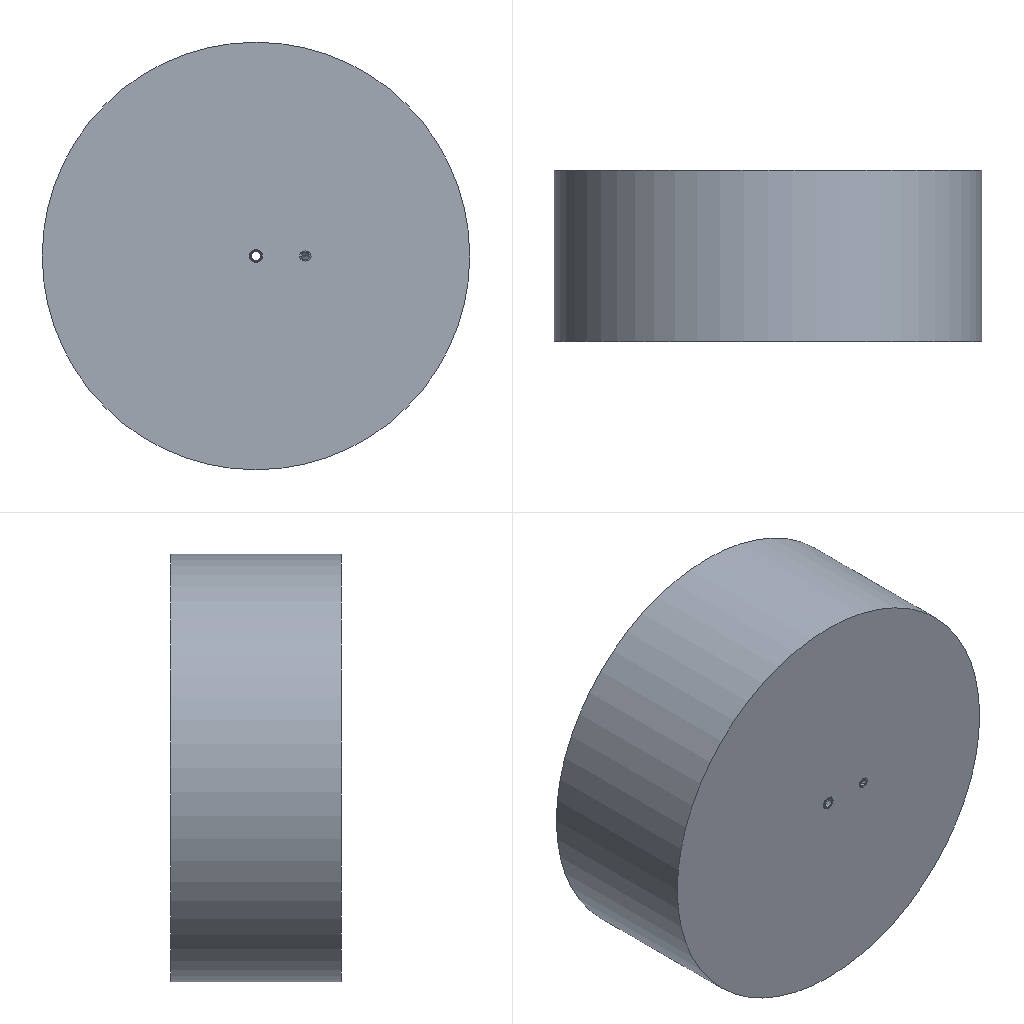Simulation study | abaqus
Set-up summary:
category,name,step,type,value,unit,region
solver,abaqus
solver,version,,,Abaqus/Standard 2020
units,not stated in the deck,,not stated
analysis,deck,,thermal,thermal
load_step,Step-1,Step-1,thermal
load_step,Step-2,Step-2,thermal
load_step,requested,,,2
mesh,nodes,,,40658
mesh,elements,,,93989
element_type,DC3D4,,solid,80589
element_type,DC3D8,,solid,13400
load,load commands in deck,,count,2
bc,support commands in deck,,count,1
material,CEMENT,,in results
material,COH,,in results
material,SOIL,,in results
material,TUBE,,in results
check,setup vs results,,match,"per instance, exact: element labels, types and connectivity; labels of the nodes the elements use; coordinates not compared"
Abaqus input file, long lists of numbers shortened:
*Heading
** Job name: TTT Model name: Model-1-Copy-Copy-TT
** Generated by: Abaqus/CAE 2020
*Preprint, echo=NO, model=NO, history=NO, contact=NO
**
** PARTS
**
*Part, name=P21
*Node
      1,   1050.777,           0.,           0.
      2,   1258.624,           0.,           0.
** (8455 more lines like these left out)
*Element, type=DC3D4
    1, 7574, 7583, 3286, 7573
    2, 7581, 3288, 3287, 3349
** (25295 more lines like these left out)
*Nset, nset=Set-1, generate
    1,  8457,     1
*Elset, elset=Set-1, generate
     1,  25297,      1
** Section: tube
*Solid Section, elset=Set-1, material=tube
,
*End Part
**
*Part, name=P22
*Node
      1,  -90.683,        4000.,   89.94
      2,           0.,        4000.,   155.24
** (1216 more lines like these left out)
*Element, type=DC3D4
   1, 1083,  994, 1100, 1016
   2, 1083, 1101,  994,  993
** (3592 more lines like these left out)
*Nset, nset=Set-1, generate
    1,  1218,     1
*Elset, elset=Set-1, generate
    1,  3594,     1
*Nset, nset=Set-2, generate
    1,  1218,     1
*Elset, elset=Set-2, generate
    1,  3594,     1
** Section: cement
*Solid Section, elset=Set-2, material=cement
,
*End Part
**
*Part, name=P23
*Node
      1,           0.,           0.,        5000.
      2,           0.,           0.,       -5000.
** (9675 more lines like these left out)
*Element, type=DC3D4
    1, 2201, 2202, 2203, 2204
    2, 2201, 2202, 2205, 2203
** (51696 more lines like these left out)
*Nset, nset=Set-1, generate
    1,  9677,     1
*Elset, elset=Set-1, generate
     1,  51698,      1
** Section: soil
*Solid Section, elset=Set-1, material=soil
,
*End Part
**
*Part, name=coh
*Node
      1,   112.261,  -48.373,           0.
      2,   121.754,   10.888,           0.
** (21304 more lines like these left out)
*Element, type=DC3D8
    1,   118,   131,   130,   176,    12,    25,    24,    70
    2,   149,   130,   131,   177,    43,    24,    25,    71
** (13398 more lines like these left out)
*Nset, nset=Set-2, generate
     1,  21306,      1
*Elset, elset=Set-2, generate
     1,  13400,      1
*Nset, nset=Set-7, generate
     1,  21306,      1
*Elset, elset=Set-7, generate
     1,  13400,      1
** Section: cement
*Solid Section, elset=Set-7, material=cement
,
*End Part
**
**
** ASSEMBLY
**
*Assembly, name=Assembly
**
*Instance, name=P21-1, part=P21
*End Instance
**
*Instance, name=P22-1, part=P22
*End Instance
**
*Instance, name=P23-1, part=P23
          0.,        4000.,           0.
          0.,        4000.,           0.,           1.,        4000., 6.12323426292584e-17,         180.
*End Instance
**
*Instance, name=coh-1, part=coh
          0.,           0.,           0.
          0.,           0.,           0., -1.,           0.,           0., 90.
*End Instance
**
*Nset, nset=Set-1, instance=P21-1
   1,   2,   3,   4,   9,  10,  11,  12,  17,  18,  19,  20,  21,  22,  23,  24
  25,  26,  27,  28,  29,  30,  31,  32,  33,  34,  35,  36,  37,  38,  39,  40
** (4 more lines like these left out)
*Nset, nset=Set-1, instance=P22-1
  10,  11,  12,  13, 135, 136, 137, 138, 139, 140, 163, 164, 165, 166, 167, 168
*Nset, nset=Set-1, instance=P23-1
    5,    6,    9,   10,   11,   12,   88,   89,   90,   91,   92,   93,  112,  113,  114,  115
  116,  117,  124,  125,  126,  127,  128,  129,  130,  131,  132,  133,  134,  135,  136,  137
** (53 more lines like these left out)
*Elset, elset=Set-1, instance=P21-1
   838,   844,   850,   902,   938,  1491,  6031, 10297, 10301, 10312, 10314, 10326, 10328, 10341, 10342, 10361
 10389, 10392, 10394, 10405, 10420, 10436, 10440, 10451, 10465, 10466, 10468, 10473, 10474, 10481, 10482, 10487
** (4 more lines like these left out)
*Elset, elset=Set-1, instance=P22-1
  137,  140,  149,  150,  172,  563,  564,  723,  740,  744,  752,  777,  789,  797,  836, 1811
*Elset, elset=Set-1, instance=P23-1
    15,   152,   213,   350,   508,   532,   550,   619,   665,   831,  1279,  1311,  1422,  1458,  1522,  1597
  1651,  1745,  1796,  1807,  1938,  2013,  2113,  2181,  2314,  2352,  2353,  2435,  2530,  2604,  2626,  2627
** (103 more lines like these left out)
*Nset, nset=Set-2, instance=P21-1, generate
    1,  8457,     1
*Nset, nset=Set-2, instance=P22-1, generate
    1,  1218,     1
*Nset, nset=Set-2, instance=P23-1, generate
    1,  9677,     1
*Elset, elset=Set-2, instance=P21-1, generate
     1,  25297,      1
*Elset, elset=Set-2, instance=P22-1, generate
    1,  3594,     1
*Elset, elset=Set-2, instance=P23-1, generate
     1,  51698,      1
*Nset, nset=Set-3, instance=P21-1, generate
    1,  8457,     1
*Nset, nset=Set-3, instance=P22-1, generate
    1,  1218,     1
*Nset, nset=Set-3, instance=P23-1, generate
    1,  9677,     1
*Elset, elset=Set-3, instance=P21-1, generate
     1,  25297,      1
*Elset, elset=Set-3, instance=P22-1, generate
    1,  3594,     1
*Elset, elset=Set-3, instance=P23-1, generate
     1,  51698,      1
*Nset, nset=Set-4, instance=P21-1, generate
    1,  8457,     1
*Nset, nset=Set-4, instance=P22-1, generate
    1,  1218,     1
*Nset, nset=Set-4, instance=P23-1, generate
    1,  9677,     1
*Elset, elset=Set-4, instance=P21-1, generate
     1,  25297,      1
*Elset, elset=Set-4, instance=P22-1, generate
    1,  3594,     1
*Elset, elset=Set-4, instance=P23-1, generate
     1,  51698,      1
*Nset, nset=Set-5, instance=P21-1, generate
    1,  8457,     1
*Nset, nset=Set-5, instance=P22-1, generate
    1,  1218,     1
*Nset, nset=Set-5, instance=P23-1, generate
    1,  9677,     1
*Nset, nset=Set-5, instance=coh-1, generate
     1,  21306,      1
*Elset, elset=Set-5, instance=P21-1, generate
     1,  25297,      1
*Elset, elset=Set-5, instance=P22-1, generate
    1,  3594,     1
*Elset, elset=Set-5, instance=P23-1, generate
     1,  51698,      1
*Elset, elset=Set-5, instance=coh-1, generate
     1,  13400,      1
*Elset, elset=_Surf-1_S3, internal, instance=P21-1
     2,     3,     8,    15,    31,    34,    47,    52,    72,    76,    84,    95,    96,   102,   110,   123
   124,   147,   149,   153,   177,   183,   185,   186,   189,   202,   206,   207,   217,   228,   235,   245
** (439 more lines like these left out)
*Elset, elset=_Surf-1_S4, internal, instance=P21-1
    29,    37,   119,   143,   154,   167,   325,   397,   465,   499,   565,   610,   652,   667,   673,   718
   773,   838,   844,   864,   913,   920,   938,   945,   955,   966,   992,  1009,  1011,  1015,  1066,  1087
** (22 more lines like these left out)
*Elset, elset=_Surf-1_S1, internal, instance=P21-1
   223,   420,   443,   459,   693,   785,   830,   866,  1608,  1623,  2301,  2526,  3215,  3218,  3593,  3598
  3692,  4192,  4402,  4443,  4547,  4582,  4586,  4798,  5314,  5372,  5657,  5929,  6073,  6639,  6643,  7053
** (13 more lines like these left out)
*Elset, elset=_Surf-1_S2, internal, instance=P21-1
    21,    54,   273,   331,   336,   367,   449,   491,   522,   543,   612,   653,   655,   658,  1065,  1111
  1139,  1180,  1261,  1290,  1705,  2255,  2774,  2778,  2863,  3034,  3327,  3662,  4244,  4304,  4344,  4485
** (16 more lines like these left out)
*Surface, type=ELEMENT, name=Surf-1
_Surf-1_S3, S3
_Surf-1_S4, S4
_Surf-1_S2, S2
_Surf-1_S1, S1
*Elset, elset=_Surf-2_S4, internal, instance=P21-1
    11,    13,    26,    29,    37,    38,    58,    59,    78,    88,    93,   112,   119,   122,   127,   143
   145,   154,   159,   167,   171,   174,   187,   190,   196,   199,   212,   243,   262,   285,   297,   300
** (158 more lines like these left out)
*Elset, elset=_Surf-2_S4, internal, instance=P22-1
   10,   13,   15,   19,   21,   29,   64,   82,   86,   93,   99,  103,  106,  110,  121,  128
  143,  156,  160,  165,  170,  174,  200,  231,  238,  243,  245,  254,  262,  263,  269,  272
** (16 more lines like these left out)
*Elset, elset=_Surf-2_S4, internal, instance=P23-1
   293,  1215,  1422,  1704,  2620,  2635,  2721,  2737,  2758,  2882,  2966,  3146,  3160,  3288,  3450,  3914
  4023,  4055,  4489,  4644,  4717,  4811,  4903,  5114,  5203,  5349,  5376,  5379,  5392,  5576,  5614,  5738
** (8 more lines like these left out)
*Elset, elset=_Surf-2_S2, internal, instance=P21-1
     1,     7,    12,    21,    23,    27,    35,    54,    56,    66,    67,    74,    77,    90,    94,    99
   105,   116,   125,   131,   134,   135,   140,   144,   156,   160,   161,   168,   178,   181,   184,   191
** (204 more lines like these left out)
*Elset, elset=_Surf-2_S2, internal, instance=P22-1
    3,   14,   26,   39,   44,   51,   53,   60,   66,   68,   72,   85,   92,  102,  104,  109
  122,  127,  129,  134,  137,  140,  144,  149,  155,  158,  172,  176,  177,  179,  189,  204
** (25 more lines like these left out)
*Elset, elset=_Surf-2_S2, internal, instance=P23-1
    15,   213,  1425,  2671,  2680,  2681,  2697,  2946,  3058,  3136,  3248,  3276,  3288,  3625,  3774,  3778
  3922,  4321,  4378,  4380,  4426,  4580,  4736,  4740,  4848,  4913,  5018,  5098,  5140,  5172,  5368,  5369
** (10 more lines like these left out)
*Elset, elset=_Surf-2_S1, internal, instance=P21-1
    17,    18,    19,    28,    42,    45,    46,    48,    57,    63,    71,    73,    79,    80,    82,    89
   100,   104,   111,   113,   117,   120,   136,   137,   150,   169,   173,   188,   193,   194,   197,   201
** (219 more lines like these left out)
*Elset, elset=_Surf-2_S1, internal, instance=P22-1
    4,    7,   20,   27,   30,   32,   33,   69,   75,   76,   77,   81,  101,  113,  116,  123
  131,  135,  137,  149,  150,  159,  163,  168,  178,  181,  182,  184,  186,  192,  201,  209
** (24 more lines like these left out)
*Elset, elset=_Surf-2_S1, internal, instance=P23-1
  2647,  2650,  2681,  2737,  4903,  5051,  5114,  5379,  5562,  5942,  5948,  5991,  6048,  6147,  6285,  6327
  6728,  6913,  7548,  7761,  7950,  7962,  8070,  8084,  8120,  8147,  8159,  8448,  8627,  8801,  8819,  8866
** (6 more lines like these left out)
*Elset, elset=_Surf-2_S3, internal, instance=P21-1
     2,     3,     8,    15,    31,    34,    47,    52,    72,    76,    84,    85,    95,    96,   102,   106
   108,   110,   123,   124,   141,   147,   149,   153,   175,   177,   183,   185,   186,   189,   202,   206
** (467 more lines like these left out)
*Elset, elset=_Surf-2_S3, internal, instance=P22-1
   24,   43,   73,  118,  164,  196,  240,  310,  343,  368,  376,  385,  406,  423,  430,  499
  564,  581,  727,  735,  752,  797,  849,  881,  956, 1048, 1196, 1213, 1256, 1265, 1315, 1330
** (3 more lines like these left out)
*Elset, elset=_Surf-2_S3, internal, instance=P23-1
    27,    30,    53,    61,    90,   113,   114,   152,   174,   210,   218,   350,   398,   498,   502,   503
   508,   532,   550,   619,   665,   741,   831,   847,   928,  1058,  1143,  1209,  1243,  1279,  1311,  1319
** (245 more lines like these left out)
*Surface, type=ELEMENT, name=Surf-2
_Surf-2_S4, S4
_Surf-2_S2, S2
_Surf-2_S1, S1
_Surf-2_S3, S3
*Elset, elset=_Surf-3_S4, internal, instance=P21-1
    11,    13,    26,    29,    37,    38,    58,    59,    78,    88,    93,   112,   119,   122,   127,   143
   145,   154,   159,   167,   171,   174,   187,   190,   196,   199,   212,   243,   262,   285,   297,   300
** (158 more lines like these left out)
*Elset, elset=_Surf-3_S4, internal, instance=P22-1
   10,   13,   15,   19,   21,   29,   64,   82,   86,   93,   99,  103,  106,  110,  121,  128
  143,  156,  160,  165,  170,  174,  200,  231,  238,  243,  245,  254,  262,  263,  269,  272
** (16 more lines like these left out)
*Elset, elset=_Surf-3_S4, internal, instance=P23-1
   293,  1215,  1422,  1704,  2620,  2635,  2721,  2737,  2758,  2882,  2966,  3146,  3160,  3288,  3450,  3914
  4023,  4055,  4489,  4644,  4717,  4811,  4903,  5114,  5203,  5349,  5376,  5379,  5392,  5576,  5614,  5738
** (8 more lines like these left out)
*Elset, elset=_Surf-3_S2, internal, instance=P21-1
     1,     7,    12,    21,    23,    27,    35,    54,    56,    66,    67,    74,    77,    90,    94,    99
   105,   116,   125,   131,   134,   135,   140,   144,   156,   160,   161,   168,   178,   181,   184,   191
** (204 more lines like these left out)
*Elset, elset=_Surf-3_S2, internal, instance=P22-1
    3,   14,   26,   39,   44,   51,   53,   60,   66,   68,   72,   85,   92,  102,  104,  109
  122,  127,  129,  134,  137,  140,  144,  149,  155,  158,  172,  176,  177,  179,  189,  204
** (25 more lines like these left out)
*Elset, elset=_Surf-3_S2, internal, instance=P23-1
    15,   213,  1425,  2671,  2680,  2681,  2697,  2946,  3058,  3136,  3248,  3276,  3288,  3625,  3774,  3778
  3922,  4321,  4378,  4380,  4426,  4580,  4736,  4740,  4848,  4913,  5018,  5098,  5140,  5172,  5368,  5369
** (10 more lines like these left out)
*Elset, elset=_Surf-3_S1, internal, instance=P21-1
    17,    18,    19,    28,    42,    45,    46,    48,    57,    63,    71,    73,    79,    80,    82,    89
   100,   104,   111,   113,   117,   120,   136,   137,   150,   169,   173,   188,   193,   194,   197,   201
** (219 more lines like these left out)
*Elset, elset=_Surf-3_S1, internal, instance=P22-1
    4,    7,   20,   27,   30,   32,   33,   69,   75,   76,   77,   81,  101,  113,  116,  123
  131,  135,  137,  149,  150,  159,  163,  168,  178,  181,  182,  184,  186,  192,  201,  209
** (24 more lines like these left out)
*Elset, elset=_Surf-3_S1, internal, instance=P23-1
  2647,  2650,  2681,  2737,  4903,  5051,  5114,  5379,  5562,  5942,  5948,  5991,  6048,  6147,  6285,  6327
  6728,  6913,  7548,  7761,  7950,  7962,  8070,  8084,  8120,  8147,  8159,  8448,  8627,  8801,  8819,  8866
** (6 more lines like these left out)
*Elset, elset=_Surf-3_S3, internal, instance=P21-1
     2,     3,     8,    15,    31,    34,    47,    52,    72,    76,    84,    85,    95,    96,   102,   106
   108,   110,   123,   124,   141,   147,   149,   153,   175,   177,   183,   185,   186,   189,   202,   206
** (467 more lines like these left out)
*Elset, elset=_Surf-3_S3, internal, instance=P22-1
   24,   43,   73,  118,  164,  196,  240,  310,  343,  368,  376,  385,  406,  423,  430,  499
  564,  581,  727,  735,  752,  797,  849,  881,  956, 1048, 1196, 1213, 1256, 1265, 1315, 1330
** (3 more lines like these left out)
*Elset, elset=_Surf-3_S3, internal, instance=P23-1
    27,    30,    53,    61,    90,   113,   114,   152,   174,   210,   218,   350,   398,   498,   502,   503
   508,   532,   550,   619,   665,   741,   831,   847,   928,  1058,  1143,  1209,  1243,  1279,  1311,  1319
** (245 more lines like these left out)
*Surface, type=ELEMENT, name=Surf-3
_Surf-3_S4, S4
_Surf-3_S2, S2
_Surf-3_S1, S1
_Surf-3_S3, S3
*Elset, elset=_Surf-14_S4, internal, instance=P21-1
    11,    13,    26,    29,    37,    38,    58,    59,    78,    88,    93,   112,   119,   122,   127,   143
   145,   154,   159,   167,   171,   174,   187,   190,   196,   199,   212,   243,   262,   285,   297,   300
** (158 more lines like these left out)
*Elset, elset=_Surf-14_S4, internal, instance=P22-1
   10,   13,   15,   19,   21,   29,   38,   47,   64,   71,   82,   86,   93,   99,  103,  106
  110,  121,  128,  143,  156,  160,  165,  166,  167,  169,  170,  174,  175,  190,  200,  207
** (25 more lines like these left out)
*Elset, elset=_Surf-14_S4, internal, instance=P23-1
   293,  1215,  1422,  1704,  2620,  2635,  2721,  2737,  2758,  2882,  2966,  3146,  3160,  3288,  3450,  3914
  4023,  4055,  4489,  4644,  4717,  4811,  4903,  5114,  5203,  5349,  5376,  5379,  5392,  5576,  5614,  5738
** (8 more lines like these left out)
*Elset, elset=_Surf-14_S4, internal, instance=coh-1
     4,     9,    10,    14,    15,    18,    19,    20,    25,    26,    30,    31,    32,    33,    39,    52
    59,    63,    64,    71,    76,    77,    81,    82,    85,    86,    87,    92,    93,    97,    98,    99
** (236 more lines like these left out)
*Elset, elset=_Surf-14_S2, internal, instance=P21-1
     1,     7,    12,    21,    23,    27,    35,    54,    56,    66,    67,    74,    77,    90,    94,    99
   105,   116,   125,   131,   134,   135,   140,   144,   156,   160,   161,   168,   178,   181,   184,   191
** (204 more lines like these left out)
*Elset, elset=_Surf-14_S2, internal, instance=P22-1
    3,   14,   18,   26,   39,   44,   51,   53,   60,   66,   68,   72,   80,   85,   92,  102
  104,  109,  122,  127,  129,  134,  137,  140,  144,  149,  155,  158,  172,  176,  177,  179
** (31 more lines like these left out)
*Elset, elset=_Surf-14_S2, internal, instance=P23-1
    15,   213,  1425,  2671,  2680,  2681,  2697,  2946,  3058,  3136,  3248,  3276,  3288,  3625,  3774,  3778
  3922,  4321,  4378,  4380,  4426,  4580,  4736,  4740,  4848,  4913,  5018,  5098,  5140,  5172,  5368,  5369
** (10 more lines like these left out)
*Elset, elset=_Surf-14_S2, internal, instance=coh-1, generate
  1,  67,   1
*Elset, elset=_Surf-14_S1, internal, instance=P21-1
    17,    18,    19,    28,    42,    45,    46,    48,    57,    63,    71,    73,    79,    80,    82,    89
   100,   104,   111,   113,   117,   120,   136,   137,   150,   169,   173,   188,   193,   194,   197,   201
** (219 more lines like these left out)
*Elset, elset=_Surf-14_S1, internal, instance=P22-1
    4,    7,   20,   27,   30,   32,   33,   63,   69,   75,   76,   77,   81,  101,  113,  116
  123,  131,  135,  137,  149,  150,  159,  163,  168,  178,  181,  182,  184,  185,  186,  192
** (29 more lines like these left out)
*Elset, elset=_Surf-14_S1, internal, instance=P23-1
  2647,  2650,  2681,  2737,  4903,  5051,  5114,  5379,  5562,  5942,  5948,  5991,  6048,  6147,  6285,  6327
  6728,  6913,  7548,  7761,  7950,  7962,  8070,  8084,  8120,  8147,  8159,  8448,  8627,  8801,  8819,  8866
** (6 more lines like these left out)
*Elset, elset=_Surf-14_S1, internal, instance=coh-1, generate
 13334,  13400,      1
*Elset, elset=_Surf-14_S3, internal, instance=P21-1
     2,     3,     8,    15,    31,    34,    47,    52,    72,    76,    84,    85,    95,    96,   102,   106
   108,   110,   123,   124,   141,   147,   149,   153,   175,   177,   183,   185,   186,   189,   202,   206
** (467 more lines like these left out)
*Elset, elset=_Surf-14_S3, internal, instance=P22-1
   24,   34,   41,   43,   52,   56,   57,   58,   65,   67,   73,   94,   95,   98,  105,  112
  118,  120,  138,  161,  164,  180,  194,  195,  196,  219,  233,  236,  240,  244,  249,  250
** (62 more lines like these left out)
*Elset, elset=_Surf-14_S3, internal, instance=P23-1
    27,    30,    53,    61,    90,   113,   114,   152,   174,   210,   218,   350,   398,   498,   502,   503
   508,   532,   550,   619,   665,   741,   831,   847,   928,  1058,  1143,  1209,  1243,  1279,  1311,  1319
** (245 more lines like these left out)
*Elset, elset=_Surf-14_S3, internal, instance=coh-1
     1,     2,     6,    11,    12,    13,    22,    34,    38,    40,    41,    42,    43,    47,    48,    53
    54,    56,    57,    68,    69,    73,    78,    79,    80,    89,   101,   105,   107,   108,   109,   110
** (236 more lines like these left out)
*Elset, elset=_Surf-14_S5, internal, instance=coh-1
     1,     2,     5,     8,    11,    12,    13,    16,    17,    27,    28,    34,    35,    36,    44,    45
    47,    48,    49,    67,    68,    69,    72,    75,    78,    79,    80,    83,    84,    94,    95,   101
** (248 more lines like these left out)
*Elset, elset=_Surf-14_S6, internal, instance=coh-1
     7,     9,    10,    14,    15,    21,    23,    24,    29,    31,    32,    33,    37,    46,    50,    51
    55,    61,    65,    66,    74,    76,    77,    81,    82,    88,    90,    91,    96,    98,    99,   100
** (248 more lines like these left out)
*Surface, type=ELEMENT, name=Surf-14
_Surf-14_S4, S4
_Surf-14_S2, S2
_Surf-14_S6, S6
_Surf-14_S1, S1
_Surf-14_S3, S3
_Surf-14_S5, S5
*Elset, elset=_Surf-15_S4, internal, instance=P21-1
    11,    13,    26,    29,    37,    38,    58,    59,    78,    88,    93,   112,   119,   122,   127,   143
   145,   154,   159,   167,   171,   174,   187,   190,   196,   199,   212,   243,   262,   285,   297,   300
** (158 more lines like these left out)
*Elset, elset=_Surf-15_S4, internal, instance=P22-1
   10,   13,   15,   19,   21,   29,   38,   47,   64,   71,   82,   86,   93,   99,  103,  106
  110,  121,  128,  143,  156,  160,  165,  166,  167,  169,  170,  174,  175,  190,  200,  207
** (25 more lines like these left out)
*Elset, elset=_Surf-15_S4, internal, instance=P23-1
   293,  1215,  1422,  1704,  2620,  2635,  2721,  2737,  2758,  2882,  2966,  3146,  3160,  3288,  3450,  3914
  4023,  4055,  4489,  4644,  4717,  4811,  4903,  5114,  5203,  5349,  5376,  5379,  5392,  5576,  5614,  5738
** (8 more lines like these left out)
*Elset, elset=_Surf-15_S4, internal, instance=coh-1
     4,     9,    10,    14,    15,    18,    19,    20,    25,    26,    30,    31,    32,    33,    39,    52
    59,    63,    64,    71,    76,    77,    81,    82,    85,    86,    87,    92,    93,    97,    98,    99
** (236 more lines like these left out)
*Elset, elset=_Surf-15_S2, internal, instance=P21-1
     1,     7,    12,    21,    23,    27,    35,    54,    56,    66,    67,    74,    77,    90,    94,    99
   105,   116,   125,   131,   134,   135,   140,   144,   156,   160,   161,   168,   178,   181,   184,   191
** (204 more lines like these left out)
*Elset, elset=_Surf-15_S2, internal, instance=P22-1
    3,   14,   18,   26,   39,   44,   51,   53,   60,   66,   68,   72,   80,   85,   92,  102
  104,  109,  122,  127,  129,  134,  137,  140,  144,  149,  155,  158,  172,  176,  177,  179
** (31 more lines like these left out)
*Elset, elset=_Surf-15_S2, internal, instance=P23-1
    15,   213,  1425,  2671,  2680,  2681,  2697,  2946,  3058,  3136,  3248,  3276,  3288,  3625,  3774,  3778
  3922,  4321,  4378,  4380,  4426,  4580,  4736,  4740,  4848,  4913,  5018,  5098,  5140,  5172,  5368,  5369
** (10 more lines like these left out)
*Elset, elset=_Surf-15_S2, internal, instance=coh-1, generate
  1,  67,   1
*Elset, elset=_Surf-15_S1, internal, instance=P21-1
    17,    18,    19,    28,    42,    45,    46,    48,    57,    63,    71,    73,    79,    80,    82,    89
   100,   104,   111,   113,   117,   120,   136,   137,   150,   169,   173,   188,   193,   194,   197,   201
** (219 more lines like these left out)
*Elset, elset=_Surf-15_S1, internal, instance=P22-1
    4,    7,   20,   27,   30,   32,   33,   63,   69,   75,   76,   77,   81,  101,  113,  116
  123,  131,  135,  137,  149,  150,  159,  163,  168,  178,  181,  182,  184,  185,  186,  192
** (29 more lines like these left out)
*Elset, elset=_Surf-15_S1, internal, instance=P23-1
  2647,  2650,  2681,  2737,  4903,  5051,  5114,  5379,  5562,  5942,  5948,  5991,  6048,  6147,  6285,  6327
  6728,  6913,  7548,  7761,  7950,  7962,  8070,  8084,  8120,  8147,  8159,  8448,  8627,  8801,  8819,  8866
** (6 more lines like these left out)
*Elset, elset=_Surf-15_S1, internal, instance=coh-1, generate
 13334,  13400,      1
*Elset, elset=_Surf-15_S3, internal, instance=P21-1
     2,     3,     8,    15,    31,    34,    47,    52,    72,    76,    84,    85,    95,    96,   102,   106
   108,   110,   123,   124,   141,   147,   149,   153,   175,   177,   183,   185,   186,   189,   202,   206
** (467 more lines like these left out)
*Elset, elset=_Surf-15_S3, internal, instance=P22-1
   24,   34,   41,   43,   52,   56,   57,   58,   65,   67,   73,   94,   95,   98,  105,  112
  118,  120,  138,  161,  164,  180,  194,  195,  196,  219,  233,  236,  240,  244,  249,  250
** (62 more lines like these left out)
*Elset, elset=_Surf-15_S3, internal, instance=P23-1
    27,    30,    53,    61,    90,   113,   114,   152,   174,   210,   218,   350,   398,   498,   502,   503
   508,   532,   550,   619,   665,   741,   831,   847,   928,  1058,  1143,  1209,  1243,  1279,  1311,  1319
** (245 more lines like these left out)
*Elset, elset=_Surf-15_S3, internal, instance=coh-1
     1,     2,     6,    11,    12,    13,    22,    34,    38,    40,    41,    42,    43,    47,    48,    53
    54,    56,    57,    68,    69,    73,    78,    79,    80,    89,   101,   105,   107,   108,   109,   110
** (236 more lines like these left out)
*Elset, elset=_Surf-15_S5, internal, instance=coh-1
     1,     2,     5,     8,    11,    12,    13,    16,    17,    27,    28,    34,    35,    36,    44,    45
    47,    48,    49,    67,    68,    69,    72,    75,    78,    79,    80,    83,    84,    94,    95,   101
** (248 more lines like these left out)
*Elset, elset=_Surf-15_S6, internal, instance=coh-1
     7,     9,    10,    14,    15,    21,    23,    24,    29,    31,    32,    33,    37,    46,    50,    51
    55,    61,    65,    66,    74,    76,    77,    81,    82,    88,    90,    91,    96,    98,    99,   100
** (248 more lines like these left out)
*Surface, type=ELEMENT, name=Surf-15
_Surf-15_S4, S4
_Surf-15_S2, S2
_Surf-15_S6, S6
_Surf-15_S1, S1
_Surf-15_S3, S3
_Surf-15_S5, S5
*Elset, elset=_m_Surf-4_S2, internal, instance=P21-1
     1,     7,    12,    23,    27,    35,    56,    66,    67,    74,    77,    90,    94,    99,   105,   116
   125,   131,   134,   135,   140,   144,   156,   160,   161,   168,   178,   181,   184,   191,   215,   216
** (137 more lines like these left out)
*Elset, elset=_m_Surf-4_S4, internal, instance=P21-1
    11,    13,    26,    38,    58,    78,    88,    93,   112,   122,   127,   145,   159,   171,   174,   187
   190,   196,   199,   212,   243,   262,   285,   297,   300,   316,   337,   344,   352,   378,   390,   404
** (90 more lines like these left out)
*Elset, elset=_m_Surf-4_S1, internal, instance=P21-1
    17,    18,    19,    28,    42,    45,    46,    48,    57,    63,    71,    73,    79,    80,    82,    89
   100,   104,   111,   113,   117,   120,   136,   137,   150,   169,   173,   188,   193,   194,   197,   201
** (148 more lines like these left out)
*Elset, elset=_m_Surf-4_S3, internal, instance=P21-1
    85,   106,   108,   141,   175,   211,   272,   345,   348,   368,   376,   417,   462,   471,   492,   498
   550,   551,   554,   564,   615,   640,   661,   682,   687,   735,   765,   803,   811,   889,   901,   915
** (17 more lines like these left out)
*Surface, type=ELEMENT, name=m_Surf-4
_m_Surf-4_S2, S2
_m_Surf-4_S4, S4
_m_Surf-4_S1, S1
_m_Surf-4_S3, S3
*Elset, elset=_m_Surf-6_S4, internal, instance=P22-1
   64,  480,  490,  496,  497,  672,  832, 1112, 1114, 1197, 1198, 1222, 1229, 1233, 1235, 1237
 1248, 1305, 1312, 1316, 1332, 1344, 1401, 1406, 1435, 1446, 1448, 1450, 1480, 1501, 1570, 1578
** (10 more lines like these left out)
*Elset, elset=_m_Surf-6_S2, internal, instance=P22-1
  102,  446,  771,  792,  923,  983, 1188, 1193, 1195, 1200, 1204, 1206, 1212, 1216, 1236, 1249
 1250, 1258, 1268, 1269, 1274, 1282, 1283, 1284, 1294, 1295, 1300, 1314, 1318, 1325, 1339, 1340
** (16 more lines like these left out)
*Elset, elset=_m_Surf-6_S3, internal, instance=P22-1
  423,  727,  849, 1196, 1256, 1265, 1315, 1330, 1343, 1752, 1758, 1792, 1884, 1888, 1892, 1895
 1936, 1947, 2008, 2011, 2226, 2297, 2342, 2357, 2565, 2574, 2575, 2586, 2587, 2610, 2632, 2688
** (1 more lines like these left out)
*Elset, elset=_m_Surf-6_S1, internal, instance=P22-1
  489,  844, 1202, 1211, 1220, 1221, 1227, 1231, 1241, 1245, 1255, 1261, 1264, 1270, 1273, 1285
 1287, 1288, 1290, 1297, 1298, 1306, 1317, 1320, 1326, 1331, 1334, 1335, 1348, 1349, 1361, 1364
** (16 more lines like these left out)
*Surface, type=ELEMENT, name=m_Surf-6
_m_Surf-6_S4, S4
_m_Surf-6_S2, S2
_m_Surf-6_S3, S3
_m_Surf-6_S1, S1
*Elset, elset=_m_Surf-8_S2, internal, instance=P21-1
     1,     7,    12,    23,    27,    35,    56,    66,    67,    74,    77,    90,    94,    99,   105,   116
   125,   131,   134,   135,   140,   144,   156,   160,   161,   168,   178,   181,   184,   191,   215,   216
** (137 more lines like these left out)
*Elset, elset=_m_Surf-8_S4, internal, instance=P21-1
    11,    13,    26,    38,    58,    78,    88,    93,   112,   122,   127,   145,   159,   171,   174,   187
   190,   196,   199,   212,   243,   262,   285,   297,   300,   316,   337,   344,   352,   378,   390,   404
** (90 more lines like these left out)
*Elset, elset=_m_Surf-8_S1, internal, instance=P21-1
    17,    18,    19,    28,    42,    45,    46,    48,    57,    63,    71,    73,    79,    80,    82,    89
   100,   104,   111,   113,   117,   120,   136,   137,   150,   169,   173,   188,   193,   194,   197,   201
** (148 more lines like these left out)
*Elset, elset=_m_Surf-8_S3, internal, instance=P21-1
    85,   106,   108,   141,   175,   211,   272,   345,   348,   368,   376,   417,   462,   471,   492,   498
   550,   551,   554,   564,   615,   640,   661,   682,   687,   735,   765,   803,   811,   889,   901,   915
** (17 more lines like these left out)
*Surface, type=ELEMENT, name=m_Surf-8
_m_Surf-8_S2, S2
_m_Surf-8_S4, S4
_m_Surf-8_S1, S1
_m_Surf-8_S3, S3
*Elset, elset=_m_Surf-10_S5, internal, instance=coh-1
     1,     5,     8,    11,    12,    13,    17,    27,    34,    49,    67,    68,    72,    75,    78,    79
    80,    84,    94,   101,   116,   134,   135,   139,   142,   145,   146,   147,   151,   161,   168,   183
** (136 more lines like these left out)
*Elset, elset=_m_Surf-10_S3, internal, instance=coh-1
     2,     6,    38,    47,    48,    56,    57,    69,    73,   105,   114,   115,   123,   124,   136,   140
   172,   181,   182,   190,   191,   203,   207,   239,   248,   249,   257,   258,   270,   274,   306,   315
** (86 more lines like these left out)
*Elset, elset=_m_Surf-10_S6, internal, instance=coh-1
     7,    10,    15,    23,    29,    31,    32,    37,    46,    51,    61,    74,    77,    82,    90,    96
    98,    99,   104,   113,   118,   128,   141,   144,   149,   157,   163,   165,   166,   171,   180,   185
** (136 more lines like these left out)
*Elset, elset=_m_Surf-10_S4, internal, instance=coh-1
     9,    14,    18,    19,    20,    26,    30,    33,    39,    52,    59,    76,    81,    85,    86,    87
    93,    97,   100,   106,   119,   126,   143,   148,   152,   153,   154,   160,   164,   167,   173,   186
** (136 more lines like these left out)
*Surface, type=ELEMENT, name=m_Surf-10
_m_Surf-10_S5, S5
_m_Surf-10_S3, S3
_m_Surf-10_S6, S6
_m_Surf-10_S4, S4
*Elset, elset=_m_Surf-12_S2, internal, instance=P21-1
     1,     7,    12,    23,    27,    35,    56,    66,    67,    74,    77,    90,    94,    99,   105,   116
   125,   131,   134,   135,   140,   144,   156,   160,   161,   168,   178,   181,   184,   191,   215,   216
** (137 more lines like these left out)
*Elset, elset=_m_Surf-12_S4, internal, instance=P21-1
    11,    13,    26,    38,    58,    78,    88,    93,   112,   122,   127,   145,   159,   171,   174,   187
   190,   196,   199,   212,   243,   262,   285,   297,   300,   316,   337,   344,   352,   378,   390,   404
** (90 more lines like these left out)
*Elset, elset=_m_Surf-12_S1, internal, instance=P21-1
    17,    18,    19,    28,    42,    45,    46,    48,    57,    63,    71,    73,    79,    80,    82,    89
   100,   104,   111,   113,   117,   120,   136,   137,   150,   169,   173,   188,   193,   194,   197,   201
** (148 more lines like these left out)
*Elset, elset=_m_Surf-12_S3, internal, instance=P21-1
    85,   106,   108,   141,   175,   211,   272,   345,   348,   368,   376,   417,   462,   471,   492,   498
   550,   551,   554,   564,   615,   640,   661,   682,   687,   735,   765,   803,   811,   889,   901,   915
** (17 more lines like these left out)
*Surface, type=ELEMENT, name=m_Surf-12
_m_Surf-12_S2, S2
_m_Surf-12_S4, S4
_m_Surf-12_S1, S1
_m_Surf-12_S3, S3
*Elset, elset=_s_Surf-6_S3, internal, instance=P23-1
   113,  2445,  2454,  2467,  2494,  2580,  2618,  2650,  2656,  2661,  2675,  2682,  2686,  2687,  2711,  2727
  2747,  2753,  2754,  2855,  2863,  2924,  2936,  3141,  3147,  3270,  3293,  3338,  3399,  3442,  3477,  3544
** (29 more lines like these left out)
*Elset, elset=_s_Surf-6_S2, internal, instance=P23-1
  2680,  3058,  3136,  3276,  6688,  6694,  7196,  7224,  7651,  7764,  7931,  7936,  7968,  8152,  8158,  8593
  9731, 11220, 11245, 11502, 16204, 17280
*Elset, elset=_s_Surf-6_S4, internal, instance=P23-1
  3160,  3288,  3450,  4055,  6539,  7704,  7827,  7836,  7940,  7977,  8310,  8312, 11229, 11293, 12046, 12974
 19345, 22350, 22855, 24051, 25027, 35622, 36049
*Elset, elset=_s_Surf-6_S1, internal, instance=P23-1
  6913,  7548,  7950,  7962,  8070,  8120,  8147,  8159,  8448, 11391, 11736, 15689, 16349, 16350, 17668, 18025
 19647, 22604, 23977, 30785, 32849, 35625, 36410, 36685, 38378
*Surface, type=ELEMENT, name=s_Surf-6
_s_Surf-6_S3, S3
_s_Surf-6_S2, S2
_s_Surf-6_S4, S4
_s_Surf-6_S1, S1
*Elset, elset=_s_Surf-8_S3, internal, instance=coh-1
     1,    11,    12,    13,    22,    34,    40,    41,    42,    43,    53,    54,    68,    78,    79,    80
    89,   101,   107,   108,   109,   110,   120,   121,   135,   145,   146,   147,   156,   168,   174,   175
** (148 more lines like these left out)
*Elset, elset=_s_Surf-8_S5, internal, instance=coh-1
     2,    16,    28,    35,    36,    44,    45,    47,    48,    69,    83,    95,   102,   103,   111,   112
   114,   115,   136,   150,   162,   169,   170,   178,   179,   181,   182,   203,   217,   229,   236,   237
** (111 more lines like these left out)
*Elset, elset=_s_Surf-8_S4, internal, instance=coh-1
     4,    10,    15,    25,    31,    32,    63,    64,    71,    77,    82,    92,    98,    99,   130,   131
   138,   144,   149,   159,   165,   166,   197,   198,   205,   211,   216,   226,   232,   233,   264,   265
** (98 more lines like these left out)
*Elset, elset=_s_Surf-8_S6, internal, instance=coh-1
     9,    14,    21,    24,    33,    50,    55,    65,    66,    76,    81,    88,    91,   100,   117,   122
   132,   133,   143,   148,   155,   158,   167,   184,   189,   199,   200,   210,   215,   222,   225,   234
** (111 more lines like these left out)
*Surface, type=ELEMENT, name=s_Surf-8
_s_Surf-8_S3, S3
_s_Surf-8_S5, S5
_s_Surf-8_S4, S4
_s_Surf-8_S6, S6
*Elset, elset=_s_Surf-10_S3, internal, instance=P22-1
  138,  332,  350,  367,  380,  415,  428,  449,  488,  570,  575,  612,  638,  669,  698,  840
  875,  891,  892,  902,  917,  934, 1022, 1072, 1079, 1081, 1136, 1156, 1210, 1219, 1223, 1267
** (37 more lines like these left out)
*Elset, elset=_s_Surf-10_S4, internal, instance=P22-1
  167,  175,  212,  619,  760,  993, 1027, 1166, 1263, 1356, 1358, 1360, 1389, 1432, 1455, 1518
 1627, 1646, 1665, 1779, 1808, 1815, 1823, 1964, 1978, 1988, 2035, 2143, 2163, 2188, 2211, 2221
** (4 more lines like these left out)
*Elset, elset=_s_Surf-10_S2, internal, instance=P22-1
  804, 1379, 1556, 1581, 1856, 1866, 1904, 1958, 1985, 2017, 2018, 2069, 2090, 2145, 2157, 2159
 2281, 2449, 2462, 2472, 2496, 2504, 2628, 2710, 2739, 2796, 2945, 2950, 2951, 3033, 3094, 3222
** (1 more lines like these left out)
*Elset, elset=_s_Surf-10_S1, internal, instance=P22-1
 1228, 1346, 1377, 1393, 1421, 1472, 1486, 1491, 1577, 1755, 1776, 1828, 1833, 1955, 1957, 1963
 2033, 2100, 2149, 2153, 2181, 2186, 2212, 2296, 2365, 2390, 2420, 2661, 2709, 2876, 2943, 3028
** (1 more lines like these left out)
*Surface, type=ELEMENT, name=s_Surf-10
_s_Surf-10_S3, S3
_s_Surf-10_S4, S4
_s_Surf-10_S2, S2
_s_Surf-10_S1, S1
*Elset, elset=_s_Surf-12_S3, internal, instance=P22-1
  138,  332,  350,  367,  380,  415,  428,  449,  488,  570,  575,  612,  638,  669,  698,  840
  875,  891,  892,  902,  917,  934, 1022, 1072, 1079, 1081, 1136, 1156, 1210, 1219, 1223, 1267
** (37 more lines like these left out)
*Elset, elset=_s_Surf-12_S4, internal, instance=P22-1
  167,  175,  212,  619,  760,  993, 1027, 1166, 1263, 1356, 1358, 1360, 1389, 1432, 1455, 1518
 1627, 1646, 1665, 1779, 1808, 1815, 1823, 1964, 1978, 1988, 2035, 2143, 2163, 2188, 2211, 2221
** (4 more lines like these left out)
*Elset, elset=_s_Surf-12_S2, internal, instance=P22-1
  804, 1379, 1556, 1581, 1856, 1866, 1904, 1958, 1985, 2017, 2018, 2069, 2090, 2145, 2157, 2159
 2281, 2449, 2462, 2472, 2496, 2504, 2628, 2710, 2739, 2796, 2945, 2950, 2951, 3033, 3094, 3222
** (1 more lines like these left out)
*Elset, elset=_s_Surf-12_S1, internal, instance=P22-1
 1228, 1346, 1377, 1393, 1421, 1472, 1486, 1491, 1577, 1755, 1776, 1828, 1833, 1955, 1957, 1963
 2033, 2100, 2149, 2153, 2181, 2186, 2212, 2296, 2365, 2390, 2420, 2661, 2709, 2876, 2943, 3028
** (1 more lines like these left out)
*Surface, type=ELEMENT, name=s_Surf-12
_s_Surf-12_S3, S3
_s_Surf-12_S4, S4
_s_Surf-12_S2, S2
_s_Surf-12_S1, S1
** Constraint: Constraint-2
*Tie, name=Constraint-2, adjust=yes
s_Surf-6, m_Surf-6
** Constraint: Constraint-3
*Tie, name=Constraint-3, adjust=yes, position tolerance=1.
m_Surf-8, s_Surf-8
** Constraint: Constraint-4
*Tie, name=Constraint-4, adjust=yes, position tolerance=1.
s_Surf-10, m_Surf-10
*End Assembly
**
** MATERIALS
**
*Material, name=cement
*Conductivity
 0.9,
*Density
 1.9e-09,
*Elastic
18000., 0.14
*Expansion
 1.05e-05,
*Specific Heat
 8.65e+08,
*Material, name=coh
*Conductivity
 0.9,
*Damage Initiation, criterion=QUADS
4.,3.,3.
*Damage Evolution, type=ENERGY
10.,
*Damage Stabilization
0.001
*Density
 1.9e-09,
*Elastic, type=TRACTION
30000.,20000.,20000.
*Specific Heat
 8.65e+08,
*Material, name=soil
*Conductivity
 2.2,
*Density
 2.3e-09,
*Elastic
17000., 0.2
*Expansion
 1.03e-05,
*Specific Heat
 8.96e+08,
*Material, name=tube
*Conductivity
45.,
*Density
 7.8e-09,
*Elastic
200000., 0.3
*Expansion
 1.22e-05,
*Specific Heat
 4.6e+08,
**
** INTERACTION PROPERTIES
**
*Surface Interaction, name=IntProp-1
1.,
*Cohesive Behavior
30000.,25000.,10000.
*Damage Initiation, criterion=MAXS
1., 2.5,  3.
*Surface Interaction, name=IntProp-2
1.,
*Friction, slip tolerance=0.005
 0.3,
*Surface Behavior, pressure-overclosure=HARD
**
** PHYSICAL CONSTANTS
**
*Physical Constants, absolute zero=-273., stefan boltzmann=5.67e-08
**
** BOUNDARY CONDITIONS
**
** Name: BC-1 Type: 对称/反对称/完全固定
*Boundary
Set-1, ENCASTRE
**
** PREDEFINED FIELDS
**
** Name: Predefined Field-1   Type: Temperature
*Initial Conditions, type=TEMPERATURE
Set-5, 50.
** ----------------------------------------------------------------
**
** STEP: Step-1
**
*Step, name=Step-1, nlgeom=NO, inc=10000
*Heat Transfer, end=PERIOD, deltmx=1000.
432., 432000., 4.32, 432000.,
**
** INTERACTIONS
**
** Interaction: Int-2
*Sradiate
Surf-14, R, 20., 0.5
** Interaction: Int-3
*Sfilm
Surf-15, F, 20., 0.005
**
** OUTPUT REQUESTS
**
*Restart, write, frequency=0
**
** FIELD OUTPUT: F-Output-1
**
*Output, field
*Node Output
NT, RFL
*Element Output, directions=YES
HFL, TEMP
*Output, history, frequency=0
*End Step
** ----------------------------------------------------------------
**
** STEP: Step-2
**
*Step, name=Step-2, nlgeom=NO
*Heat Transfer, end=PERIOD, deltmx=1000.
3456., 345600., 3.456, 345600.,
**
** OUTPUT REQUESTS
**
*Restart, write, frequency=0
**
** FIELD OUTPUT: F-Output-1
**
*Output, field
*Node Output
NT, RFL
*Element Output, directions=YES
HFL, TEMP
*Output, history, frequency=0
*End Step
Results summary:
result,step,,partial,increments=0 time=0.0/432000.0
result,step,,partial,increments=0 time=0.0/345600.0
result,analysis,,,"heat transfer, deltamx"
result,last_loadstep,,,2
result,primary field,,,NT11